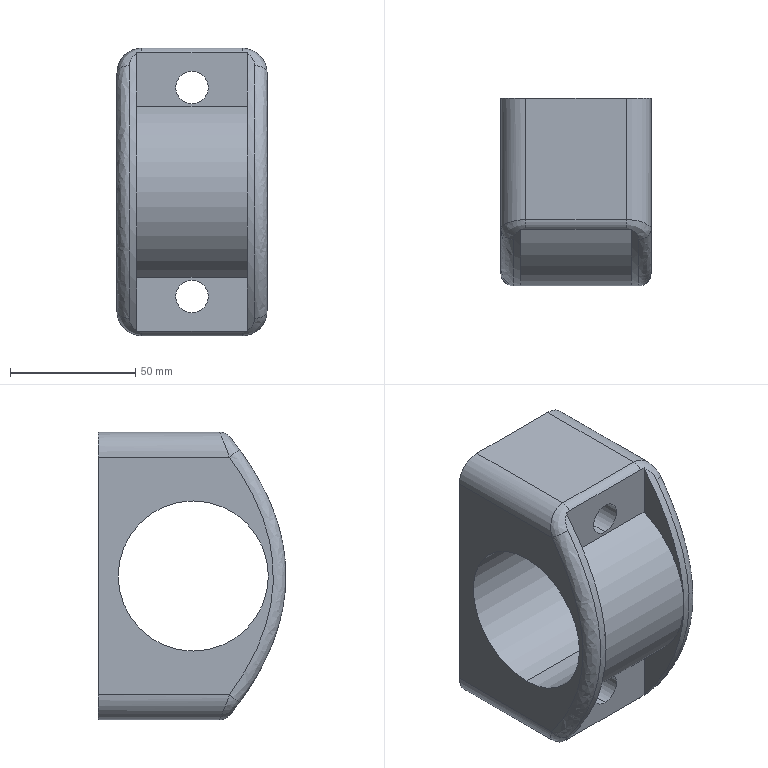Part | STEP file | Cable clamp | 1 solid | 32 faces | box 60 x 75 x 115 mm | volume 247927 mm3 | cylinder 13 | plane 11 | spline 8 | commonest cylinder face diameters 13 x4 20 x4 10 x2 60 x2 74 x1